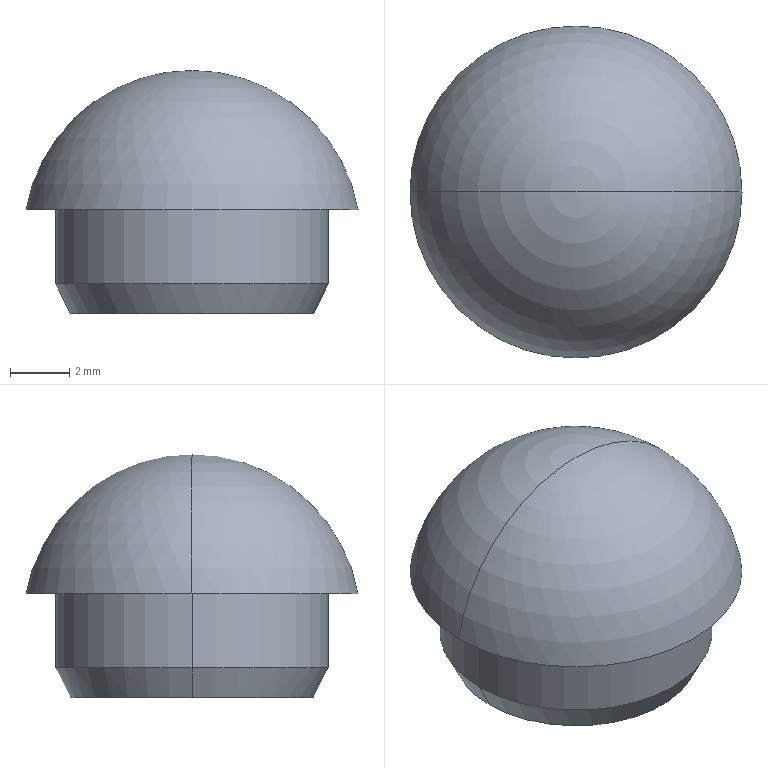Part | SolidWorks | features BaseBody 1 | 1 solid | 12 faces | box 11.2 x 11.2 x 8.2 mm | volume 267.23 mm3 | sphere 4 | cylinder 4 | plane 2 | cone 2 | commonest cylinder face diameters 7.8 x2 9.2 x2
STEP:
#1=CARTESIAN_POINT('',(-299.676,-272.746,365.447));
#2=VERTEX_POINT('',#1);
#3=CARTESIAN_POINT('',(-291.876,-272.746,365.447));
#4=VERTEX_POINT('',#3);
#5=CARTESIAN_POINT('',(-295.776,-272.746,365.447));
#6=DIRECTION('',(0.,0.,1.));
#7=DIRECTION('',(-1.,0.,0.));
#8=AXIS2_PLACEMENT_3D('',#5,#6,#7);
#9=CIRCLE('',#8,3.9);
#10=EDGE_CURVE('',#2,#4,#9,.T.);
#11=ORIENTED_EDGE('',*,*,#10,.F.);
#12=CARTESIAN_POINT('',(-295.776,-272.746,365.447));
#13=DIRECTION('',(0.,-1.,0.));
#14=DIRECTION('',(0.,0.,1.));
#15=AXIS2_PLACEMENT_3D('',#12,#13,#14);
#16=CIRCLE('',#15,3.9);
#17=EDGE_CURVE('',#4,#2,#16,.T.);
#18=ORIENTED_EDGE('',*,*,#17,.F.);
#19=EDGE_LOOP('',(#11,#18));
#20=FACE_OUTER_BOUND('',#19,.T.);
#21=CARTESIAN_POINT('',(-295.776,-272.746,365.447));
#22=DIRECTION('',(0.,0.,1.));
#23=DIRECTION('',(-1.,0.,0.));
#24=AXIS2_PLACEMENT_3D('',#21,#22,#23);
#25=SPHERICAL_SURFACE('',#24,3.9);
#26=ADVANCED_FACE('',(#20),#25,.F.);
#27=ORIENTED_EDGE('',*,*,#17,.T.);
#28=CARTESIAN_POINT('',(-295.776,-272.746,365.447));
#29=DIRECTION('',(0.,0.,1.));
#30=DIRECTION('',(1.,0.,0.));
#31=AXIS2_PLACEMENT_3D('',#28,#29,#30);
#32=CIRCLE('',#31,3.9);
#33=EDGE_CURVE('',#4,#2,#32,.T.);
#34=ORIENTED_EDGE('',*,*,#33,.F.);
#35=EDGE_LOOP('',(#27,#34));
#36=FACE_OUTER_BOUND('',#35,.T.);
#37=CARTESIAN_POINT('',(-295.776,-272.746,365.447));
#38=DIRECTION('',(0.,0.,1.));
#39=DIRECTION('',(-1.,0.,0.));
#40=AXIS2_PLACEMENT_3D('',#37,#38,#39);
#41=SPHERICAL_SURFACE('',#40,3.9);
#42=ADVANCED_FACE('',(#36),#41,.F.);
#43=ORIENTED_EDGE('',*,*,#33,.T.);
#44=CARTESIAN_POINT('',(-299.676,-272.746,362.934));
#45=VERTEX_POINT('',#44);
#46=CARTESIAN_POINT('',(-299.676,-272.746,365.447));
#47=DIRECTION('',(0.,0.,-1.));
#48=VECTOR('',#47,1000.);
#49=LINE('',#46,#48);
#50=EDGE_CURVE('',#2,#45,#49,.T.);
#51=ORIENTED_EDGE('',*,*,#50,.T.);
#52=CARTESIAN_POINT('',(-291.876,-272.746,362.934));
#53=VERTEX_POINT('',#52);
#54=CARTESIAN_POINT('',(-295.776,-272.746,362.934));
#55=DIRECTION('',(0.,0.,-1.));
#56=DIRECTION('',(-1.,0.,0.));
#57=AXIS2_PLACEMENT_3D('',#54,#55,#56);
#58=CIRCLE('',#57,3.9);
#59=EDGE_CURVE('',#45,#53,#58,.T.);
#60=ORIENTED_EDGE('',*,*,#59,.T.);
#61=CARTESIAN_POINT('',(-291.876,-272.746,365.447));
#62=DIRECTION('',(0.,0.,-1.));
#63=VECTOR('',#62,1000.);
#64=LINE('',#61,#63);
#65=EDGE_CURVE('',#4,#53,#64,.T.);
#66=ORIENTED_EDGE('',*,*,#65,.F.);
#67=EDGE_LOOP('',(#43,#51,#60,#66));
#68=FACE_OUTER_BOUND('',#67,.T.);
#69=CARTESIAN_POINT('',(-295.776,-272.746,371.544));
#70=DIRECTION('',(0.,0.,-1.));
#71=DIRECTION('',(-1.,0.,0.));
#72=AXIS2_PLACEMENT_3D('',#69,#70,#71);
#73=CYLINDRICAL_SURFACE('',#72,3.9);
#74=ADVANCED_FACE('',(#68),#73,.F.);
#75=CARTESIAN_POINT('',(-295.776,-272.746,362.934));
#76=DIRECTION('',(0.,0.,-1.));
#77=DIRECTION('',(1.,0.,0.));
#78=AXIS2_PLACEMENT_3D('',#75,#76,#77);
#79=CIRCLE('',#78,3.9);
#80=EDGE_CURVE('',#53,#45,#79,.T.);
#81=ORIENTED_EDGE('',*,*,#80,.T.);
#82=ORIENTED_EDGE('',*,*,#50,.F.);
#83=ORIENTED_EDGE('',*,*,#10,.T.);
#84=ORIENTED_EDGE('',*,*,#65,.T.);
#85=EDGE_LOOP('',(#81,#82,#83,#84));
#86=FACE_OUTER_BOUND('',#85,.T.);
#87=CARTESIAN_POINT('',(-295.776,-272.746,371.544));
#88=DIRECTION('',(0.,0.,-1.));
#89=DIRECTION('',(-1.,0.,0.));
#90=AXIS2_PLACEMENT_3D('',#87,#88,#89);
#91=CYLINDRICAL_SURFACE('',#90,3.9);
#92=ADVANCED_FACE('',(#86),#91,.F.);
#93=ORIENTED_EDGE('',*,*,#59,.F.);
#94=ORIENTED_EDGE('',*,*,#80,.F.);
#95=EDGE_LOOP('',(#93,#94));
#96=FACE_BOUND('',#95,.T.);
#97=CARTESIAN_POINT('',(-299.876,-272.746,362.934));
#98=VERTEX_POINT('',#97);
#99=CARTESIAN_POINT('',(-291.676,-272.746,362.934));
#100=VERTEX_POINT('',#99);
#101=CARTESIAN_POINT('',(-295.776,-272.746,362.934));
#102=DIRECTION('',(0.,0.,1.));
#103=DIRECTION('',(-1.,0.,0.));
#104=AXIS2_PLACEMENT_3D('',#101,#102,#103);
#105=CIRCLE('',#104,4.1);
#106=EDGE_CURVE('',#98,#100,#105,.T.);
#107=ORIENTED_EDGE('',*,*,#106,.F.);
#108=CARTESIAN_POINT('',(-295.776,-272.746,362.934));
#109=DIRECTION('',(0.,0.,1.));
#110=DIRECTION('',(1.,0.,0.));
#111=AXIS2_PLACEMENT_3D('',#108,#109,#110);
#112=CIRCLE('',#111,4.1);
#113=EDGE_CURVE('',#100,#98,#112,.T.);
#114=ORIENTED_EDGE('',*,*,#113,.F.);
#115=EDGE_LOOP('',(#107,#114));
#116=FACE_OUTER_BOUND('',#115,.T.);
#117=CARTESIAN_POINT('',(-295.776,-272.746,362.934));
#118=DIRECTION('',(0.,0.,-1.));
#119=DIRECTION('',(0.,-1.,0.));
#120=AXIS2_PLACEMENT_3D('',#117,#118,#119);
#121=PLANE('',#120);
#122=ADVANCED_FACE('',(#96,#116),#121,.T.);
#123=ORIENTED_EDGE('',*,*,#113,.T.);
#124=CARTESIAN_POINT('',(-300.376,-272.746,363.934));
#125=VERTEX_POINT('',#124);
#126=CARTESIAN_POINT('',(-299.876,-272.746,362.934));
#127=DIRECTION('',(-0.4472,0.,0.8944));
#128=VECTOR('',#127,1000.);
#129=LINE('',#126,#128);
#130=EDGE_CURVE('',#98,#125,#129,.T.);
#131=ORIENTED_EDGE('',*,*,#130,.T.);
#132=CARTESIAN_POINT('',(-291.176,-272.746,363.934));
#133=VERTEX_POINT('',#132);
#134=CARTESIAN_POINT('',(-295.776,-272.746,363.934));
#135=DIRECTION('',(0.,0.,1.));
#136=DIRECTION('',(1.,0.,0.));
#137=AXIS2_PLACEMENT_3D('',#134,#135,#136);
#138=CIRCLE('',#137,4.6);
#139=EDGE_CURVE('',#133,#125,#138,.T.);
#140=ORIENTED_EDGE('',*,*,#139,.F.);
#141=CARTESIAN_POINT('',(-291.676,-272.746,362.934));
#142=DIRECTION('',(0.4472,0.,0.8944));
#143=VECTOR('',#142,1000.);
#144=LINE('',#141,#143);
#145=EDGE_CURVE('',#100,#133,#144,.T.);
#146=ORIENTED_EDGE('',*,*,#145,.F.);
#147=EDGE_LOOP('',(#123,#131,#140,#146));
#148=FACE_OUTER_BOUND('',#147,.T.);
#149=CARTESIAN_POINT('',(-295.776,-272.746,363.434));
#150=DIRECTION('',(0.,0.,1.));
#151=DIRECTION('',(1.,0.,0.));
#152=AXIS2_PLACEMENT_3D('',#149,#150,#151);
#153=CONICAL_SURFACE('',#152,4.35,0.4636);
#154=ADVANCED_FACE('',(#148),#153,.T.);
#155=CARTESIAN_POINT('',(-295.776,-272.746,363.934));
#156=DIRECTION('',(0.,0.,1.));
#157=DIRECTION('',(-1.,0.,0.));
#158=AXIS2_PLACEMENT_3D('',#155,#156,#157);
#159=CIRCLE('',#158,4.6);
#160=EDGE_CURVE('',#125,#133,#159,.T.);
#161=ORIENTED_EDGE('',*,*,#160,.F.);
#162=ORIENTED_EDGE('',*,*,#130,.F.);
#163=ORIENTED_EDGE('',*,*,#106,.T.);
#164=ORIENTED_EDGE('',*,*,#145,.T.);
#165=EDGE_LOOP('',(#161,#162,#163,#164));
#166=FACE_OUTER_BOUND('',#165,.T.);
#167=CARTESIAN_POINT('',(-295.776,-272.746,363.434));
#168=DIRECTION('',(0.,0.,1.));
#169=DIRECTION('',(1.,0.,0.));
#170=AXIS2_PLACEMENT_3D('',#167,#168,#169);
#171=CONICAL_SURFACE('',#170,4.35,0.4636);
#172=ADVANCED_FACE('',(#166),#171,.T.);
#173=CARTESIAN_POINT('',(-291.176,-272.746,366.434));
#174=VERTEX_POINT('',#173);
#175=CARTESIAN_POINT('',(-300.376,-272.746,366.434));
#176=VERTEX_POINT('',#175);
#177=CARTESIAN_POINT('',(-295.776,-272.746,366.434));
#178=DIRECTION('',(0.,0.,-1.));
#179=DIRECTION('',(1.,0.,0.));
#180=AXIS2_PLACEMENT_3D('',#177,#178,#179);
#181=CIRCLE('',#180,4.6);
#182=EDGE_CURVE('',#174,#176,#181,.T.);
#183=ORIENTED_EDGE('',*,*,#182,.T.);
#184=CARTESIAN_POINT('',(-300.376,-272.746,363.934));
#185=DIRECTION('',(0.,0.,1.));
#186=VECTOR('',#185,1000.);
#187=LINE('',#184,#186);
#188=EDGE_CURVE('',#125,#176,#187,.T.);
#189=ORIENTED_EDGE('',*,*,#188,.F.);
#190=ORIENTED_EDGE('',*,*,#160,.T.);
#191=CARTESIAN_POINT('',(-291.176,-272.746,363.934));
#192=DIRECTION('',(0.,0.,1.));
#193=VECTOR('',#192,1000.);
#194=LINE('',#191,#193);
#195=EDGE_CURVE('',#133,#174,#194,.T.);
#196=ORIENTED_EDGE('',*,*,#195,.T.);
#197=EDGE_LOOP('',(#183,#189,#190,#196));
#198=FACE_OUTER_BOUND('',#197,.T.);
#199=CARTESIAN_POINT('',(-295.776,-272.746,371.544));
#200=DIRECTION('',(0.,0.,-1.));
#201=DIRECTION('',(-1.,0.,0.));
#202=AXIS2_PLACEMENT_3D('',#199,#200,#201);
#203=CYLINDRICAL_SURFACE('',#202,4.6);
#204=ADVANCED_FACE('',(#198),#203,.T.);
#205=ORIENTED_EDGE('',*,*,#139,.T.);
#206=ORIENTED_EDGE('',*,*,#188,.T.);
#207=CARTESIAN_POINT('',(-295.776,-272.746,366.434));
#208=DIRECTION('',(0.,0.,-1.));
#209=DIRECTION('',(-1.,0.,0.));
#210=AXIS2_PLACEMENT_3D('',#207,#208,#209);
#211=CIRCLE('',#210,4.6);
#212=EDGE_CURVE('',#176,#174,#211,.T.);
#213=ORIENTED_EDGE('',*,*,#212,.T.);
#214=ORIENTED_EDGE('',*,*,#195,.F.);
#215=EDGE_LOOP('',(#205,#206,#213,#214));
#216=FACE_OUTER_BOUND('',#215,.T.);
#217=CARTESIAN_POINT('',(-295.776,-272.746,371.544));
#218=DIRECTION('',(0.,0.,-1.));
#219=DIRECTION('',(-1.,0.,0.));
#220=AXIS2_PLACEMENT_3D('',#217,#218,#219);
#221=CYLINDRICAL_SURFACE('',#220,4.6);
#222=ADVANCED_FACE('',(#216),#221,.T.);
#223=ORIENTED_EDGE('',*,*,#212,.F.);
#224=ORIENTED_EDGE('',*,*,#182,.F.);
#225=EDGE_LOOP('',(#223,#224));
#226=FACE_BOUND('',#225,.T.);
#227=CARTESIAN_POINT('',(-301.376,-272.746,366.434));
#228=VERTEX_POINT('',#227);
#229=CARTESIAN_POINT('',(-290.176,-272.746,366.434));
#230=VERTEX_POINT('',#229);
#231=CARTESIAN_POINT('',(-295.776,-272.746,366.434));
#232=DIRECTION('',(0.,0.,1.));
#233=DIRECTION('',(-1.,0.,0.));
#234=AXIS2_PLACEMENT_3D('',#231,#232,#233);
#235=CIRCLE('',#234,5.6);
#236=EDGE_CURVE('',#228,#230,#235,.T.);
#237=ORIENTED_EDGE('',*,*,#236,.F.);
#238=CARTESIAN_POINT('',(-295.776,-272.746,366.434));
#239=DIRECTION('',(0.,0.,1.));
#240=DIRECTION('',(1.,0.,0.));
#241=AXIS2_PLACEMENT_3D('',#238,#239,#240);
#242=CIRCLE('',#241,5.6);
#243=EDGE_CURVE('',#230,#228,#242,.T.);
#244=ORIENTED_EDGE('',*,*,#243,.F.);
#245=EDGE_LOOP('',(#237,#244));
#246=FACE_OUTER_BOUND('',#245,.T.);
#247=CARTESIAN_POINT('',(-295.776,-272.746,366.434));
#248=DIRECTION('',(0.,0.,-1.));
#249=DIRECTION('',(0.,-1.,0.));
#250=AXIS2_PLACEMENT_3D('',#247,#248,#249);
#251=PLANE('',#250);
#252=ADVANCED_FACE('',(#226,#246),#251,.T.);
#253=ORIENTED_EDGE('',*,*,#243,.T.);
#254=CARTESIAN_POINT('',(-295.776,-272.746,365.447));
#255=DIRECTION('',(0.,1.,0.));
#256=DIRECTION('',(-0.9848,0.,0.1734));
#257=AXIS2_PLACEMENT_3D('',#254,#255,#256);
#258=CIRCLE('',#257,5.686);
#259=EDGE_CURVE('',#228,#230,#258,.T.);
#260=ORIENTED_EDGE('',*,*,#259,.T.);
#261=EDGE_LOOP('',(#253,#260));
#262=FACE_OUTER_BOUND('',#261,.T.);
#263=CARTESIAN_POINT('',(-295.776,-272.746,365.447));
#264=DIRECTION('',(0.,0.,1.));
#265=DIRECTION('',(-1.,0.,0.));
#266=AXIS2_PLACEMENT_3D('',#263,#264,#265);
#267=SPHERICAL_SURFACE('',#266,5.686);
#268=ADVANCED_FACE('',(#262),#267,.T.);
#269=ORIENTED_EDGE('',*,*,#259,.F.);
#270=ORIENTED_EDGE('',*,*,#236,.T.);
#271=EDGE_LOOP('',(#269,#270));
#272=FACE_OUTER_BOUND('',#271,.T.);
#273=CARTESIAN_POINT('',(-295.776,-272.746,365.447));
#274=DIRECTION('',(0.,0.,1.));
#275=DIRECTION('',(-1.,0.,0.));
#276=AXIS2_PLACEMENT_3D('',#273,#274,#275);
#277=SPHERICAL_SURFACE('',#276,5.686);
#278=ADVANCED_FACE('',(#272),#277,.T.);
#279=CLOSED_SHELL('',(#26,#42,#74,#92,#122,#154,#172,#204,#222,#252,#268,#278));
#280=MANIFOLD_SOLID_BREP('',#279);
#281=CARTESIAN_POINT('',(0.,0.,0.));
#282=DIRECTION('',(0.,0.,1.));
#283=DIRECTION('',(1.,0.,0.));
#284=AXIS2_PLACEMENT_3D('',#281,#282,#283);
#285=(LENGTH_UNIT()NAMED_UNIT(*)SI_UNIT(.MILLI.,.METRE.));
#286=UNCERTAINTY_MEASURE_WITH_UNIT(LENGTH_MEASURE(0.00001),#285,'','');
#287=(NAMED_UNIT(*)PLANE_ANGLE_UNIT()SI_UNIT($,.RADIAN.));
#288=(NAMED_UNIT(*)SI_UNIT($,.STERADIAN.)SOLID_ANGLE_UNIT());
#289=(GEOMETRIC_REPRESENTATION_CONTEXT(3)GLOBAL_UNCERTAINTY_ASSIGNED_CONTEXT((#286))GLOBAL_UNIT_ASSIGNED_CONTEXT((#285,#287,#288))REPRESENTATION_CONTEXT('',''));
#290=ADVANCED_BREP_SHAPE_REPRESENTATION('',(#280,#284),#289);